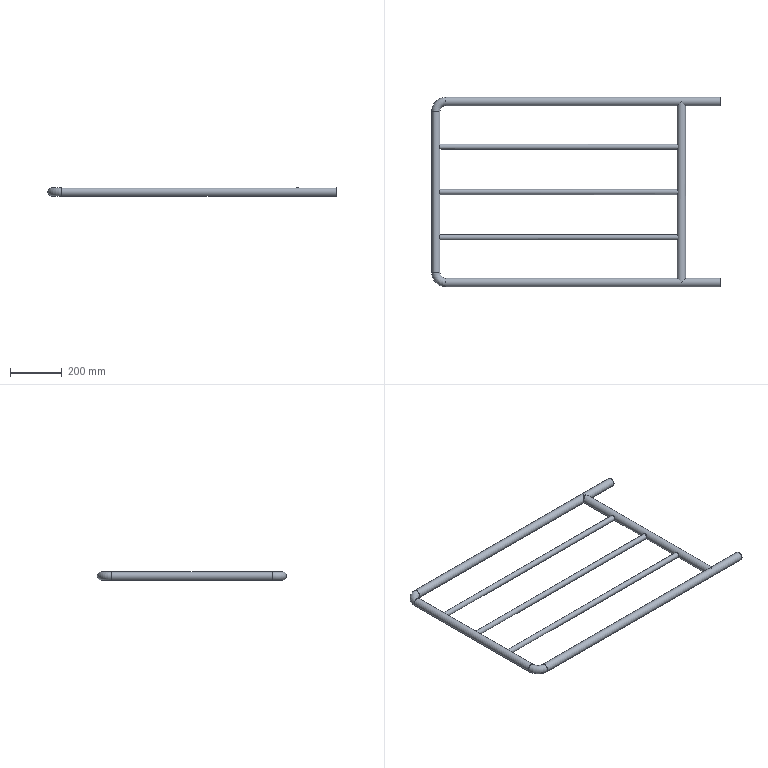Part | STEP file | 304 guardrail 700X1100 body_Default<As Machined> | 9 solids | 36 faces | box 1116 x 732 x 32 mm | volume 674327 mm3 | cylinder 22 | plane 10 | torus 4 | commonest cylinder face diameters 32 x12 29 x4 18 x3 20 x3